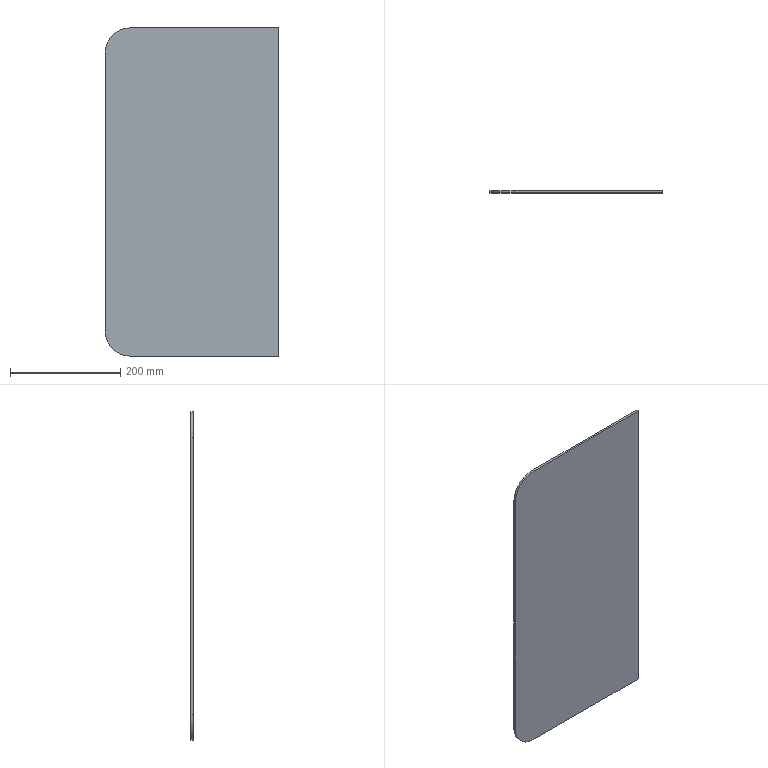Part | SolidWorks | features Extrusion 1 | 1 solid | 8 faces | box 315.5 x 4 x 596 mm | volume 748519 mm3 | plane 6 | cylinder 2 | commonest cylinder face diameters 92 x2
STEP:
#1=CARTESIAN_POINT('',(0.,0.,298.));
#2=VERTEX_POINT('',#1);
#3=CARTESIAN_POINT('',(0.,0.,-298.));
#4=VERTEX_POINT('',#3);
#5=CARTESIAN_POINT('',(0.,0.,-298.));
#6=DIRECTION('',(0.,0.,-1.));
#7=VECTOR('',#6,1000.);
#8=LINE('',#5,#7);
#9=EDGE_CURVE('',#2,#4,#8,.T.);
#10=ORIENTED_EDGE('',*,*,#9,.T.);
#11=CARTESIAN_POINT('',(0.,4.,-298.));
#12=VERTEX_POINT('',#11);
#13=CARTESIAN_POINT('',(0.,4.,-298.));
#14=DIRECTION('',(0.,-1.,0.));
#15=VECTOR('',#14,1000.);
#16=LINE('',#13,#15);
#17=EDGE_CURVE('',#12,#4,#16,.T.);
#18=ORIENTED_EDGE('',*,*,#17,.F.);
#19=CARTESIAN_POINT('',(0.,4.,298.));
#20=VERTEX_POINT('',#19);
#21=CARTESIAN_POINT('',(0.,4.,-298.));
#22=DIRECTION('',(0.,0.,-1.));
#23=VECTOR('',#22,1000.);
#24=LINE('',#21,#23);
#25=EDGE_CURVE('',#20,#12,#24,.T.);
#26=ORIENTED_EDGE('',*,*,#25,.F.);
#27=CARTESIAN_POINT('',(0.,4.,298.));
#28=DIRECTION('',(0.,-1.,0.));
#29=VECTOR('',#28,1000.);
#30=LINE('',#27,#29);
#31=EDGE_CURVE('',#20,#2,#30,.T.);
#32=ORIENTED_EDGE('',*,*,#31,.T.);
#33=EDGE_LOOP('',(#10,#18,#26,#32));
#34=FACE_OUTER_BOUND('',#33,.T.);
#35=CARTESIAN_POINT('',(0.,4.,-298.));
#36=DIRECTION('',(-1.,0.,0.));
#37=DIRECTION('',(0.,0.,1.));
#38=AXIS2_PLACEMENT_3D('',#35,#36,#37);
#39=PLANE('',#38);
#40=ADVANCED_FACE('',(#34),#39,.F.);
#41=CARTESIAN_POINT('',(-269.5,0.,-298.));
#42=VERTEX_POINT('',#41);
#43=CARTESIAN_POINT('',(0.,0.,-298.));
#44=DIRECTION('',(-1.,0.,0.));
#45=VECTOR('',#44,1000.);
#46=LINE('',#43,#45);
#47=EDGE_CURVE('',#4,#42,#46,.T.);
#48=ORIENTED_EDGE('',*,*,#47,.T.);
#49=CARTESIAN_POINT('',(-269.5,4.,-298.));
#50=VERTEX_POINT('',#49);
#51=CARTESIAN_POINT('',(-269.5,4.,-298.));
#52=DIRECTION('',(0.,-1.,0.));
#53=VECTOR('',#52,1000.);
#54=LINE('',#51,#53);
#55=EDGE_CURVE('',#50,#42,#54,.T.);
#56=ORIENTED_EDGE('',*,*,#55,.F.);
#57=CARTESIAN_POINT('',(0.,4.,-298.));
#58=DIRECTION('',(-1.,0.,0.));
#59=VECTOR('',#58,1000.);
#60=LINE('',#57,#59);
#61=EDGE_CURVE('',#12,#50,#60,.T.);
#62=ORIENTED_EDGE('',*,*,#61,.F.);
#63=ORIENTED_EDGE('',*,*,#17,.T.);
#64=EDGE_LOOP('',(#48,#56,#62,#63));
#65=FACE_OUTER_BOUND('',#64,.T.);
#66=CARTESIAN_POINT('',(0.,4.,-298.));
#67=DIRECTION('',(0.,0.,1.));
#68=DIRECTION('',(1.,0.,0.));
#69=AXIS2_PLACEMENT_3D('',#66,#67,#68);
#70=PLANE('',#69);
#71=ADVANCED_FACE('',(#65),#70,.F.);
#72=CARTESIAN_POINT('',(-315.5,0.,-252.));
#73=VERTEX_POINT('',#72);
#74=CARTESIAN_POINT('',(-269.5,0.,-252.));
#75=DIRECTION('',(0.,1.,0.));
#76=DIRECTION('',(0.,0.,1.));
#77=AXIS2_PLACEMENT_3D('',#74,#75,#76);
#78=CIRCLE('',#77,46.);
#79=EDGE_CURVE('',#42,#73,#78,.T.);
#80=ORIENTED_EDGE('',*,*,#79,.T.);
#81=CARTESIAN_POINT('',(-315.5,4.,-252.));
#82=VERTEX_POINT('',#81);
#83=CARTESIAN_POINT('',(-315.5,4.,-252.));
#84=DIRECTION('',(0.,-1.,0.));
#85=VECTOR('',#84,1000.);
#86=LINE('',#83,#85);
#87=EDGE_CURVE('',#82,#73,#86,.T.);
#88=ORIENTED_EDGE('',*,*,#87,.F.);
#89=CARTESIAN_POINT('',(-269.5,4.,-252.));
#90=DIRECTION('',(0.,1.,0.));
#91=DIRECTION('',(0.,0.,1.));
#92=AXIS2_PLACEMENT_3D('',#89,#90,#91);
#93=CIRCLE('',#92,46.);
#94=EDGE_CURVE('',#50,#82,#93,.T.);
#95=ORIENTED_EDGE('',*,*,#94,.F.);
#96=ORIENTED_EDGE('',*,*,#55,.T.);
#97=EDGE_LOOP('',(#80,#88,#95,#96));
#98=FACE_OUTER_BOUND('',#97,.T.);
#99=CARTESIAN_POINT('',(-269.5,4.,-252.));
#100=DIRECTION('',(0.,-1.,0.));
#101=DIRECTION('',(0.,0.,-1.));
#102=AXIS2_PLACEMENT_3D('',#99,#100,#101);
#103=CYLINDRICAL_SURFACE('',#102,46.);
#104=ADVANCED_FACE('',(#98),#103,.T.);
#105=CARTESIAN_POINT('',(-315.5,0.,252.));
#106=VERTEX_POINT('',#105);
#107=CARTESIAN_POINT('',(-315.5,0.,-252.));
#108=DIRECTION('',(0.,0.,1.));
#109=VECTOR('',#108,1000.);
#110=LINE('',#107,#109);
#111=EDGE_CURVE('',#73,#106,#110,.T.);
#112=ORIENTED_EDGE('',*,*,#111,.T.);
#113=CARTESIAN_POINT('',(-315.5,4.,252.));
#114=VERTEX_POINT('',#113);
#115=CARTESIAN_POINT('',(-315.5,4.,252.));
#116=DIRECTION('',(0.,-1.,0.));
#117=VECTOR('',#116,1000.);
#118=LINE('',#115,#117);
#119=EDGE_CURVE('',#114,#106,#118,.T.);
#120=ORIENTED_EDGE('',*,*,#119,.F.);
#121=CARTESIAN_POINT('',(-315.5,4.,-252.));
#122=DIRECTION('',(0.,0.,1.));
#123=VECTOR('',#122,1000.);
#124=LINE('',#121,#123);
#125=EDGE_CURVE('',#82,#114,#124,.T.);
#126=ORIENTED_EDGE('',*,*,#125,.F.);
#127=ORIENTED_EDGE('',*,*,#87,.T.);
#128=EDGE_LOOP('',(#112,#120,#126,#127));
#129=FACE_OUTER_BOUND('',#128,.T.);
#130=CARTESIAN_POINT('',(-315.5,4.,-252.));
#131=DIRECTION('',(1.,0.,0.));
#132=DIRECTION('',(0.,0.,-1.));
#133=AXIS2_PLACEMENT_3D('',#130,#131,#132);
#134=PLANE('',#133);
#135=ADVANCED_FACE('',(#129),#134,.F.);
#136=CARTESIAN_POINT('',(-269.5,0.,298.));
#137=VERTEX_POINT('',#136);
#138=CARTESIAN_POINT('',(-269.5,0.,252.));
#139=DIRECTION('',(0.,1.,0.));
#140=DIRECTION('',(0.,0.,1.));
#141=AXIS2_PLACEMENT_3D('',#138,#139,#140);
#142=CIRCLE('',#141,46.);
#143=EDGE_CURVE('',#106,#137,#142,.T.);
#144=ORIENTED_EDGE('',*,*,#143,.T.);
#145=CARTESIAN_POINT('',(-269.5,4.,298.));
#146=VERTEX_POINT('',#145);
#147=CARTESIAN_POINT('',(-269.5,4.,298.));
#148=DIRECTION('',(0.,-1.,0.));
#149=VECTOR('',#148,1000.);
#150=LINE('',#147,#149);
#151=EDGE_CURVE('',#146,#137,#150,.T.);
#152=ORIENTED_EDGE('',*,*,#151,.F.);
#153=CARTESIAN_POINT('',(-269.5,4.,252.));
#154=DIRECTION('',(0.,1.,0.));
#155=DIRECTION('',(0.,0.,1.));
#156=AXIS2_PLACEMENT_3D('',#153,#154,#155);
#157=CIRCLE('',#156,46.);
#158=EDGE_CURVE('',#114,#146,#157,.T.);
#159=ORIENTED_EDGE('',*,*,#158,.F.);
#160=ORIENTED_EDGE('',*,*,#119,.T.);
#161=EDGE_LOOP('',(#144,#152,#159,#160));
#162=FACE_OUTER_BOUND('',#161,.T.);
#163=CARTESIAN_POINT('',(-269.5,4.,252.));
#164=DIRECTION('',(0.,-1.,0.));
#165=DIRECTION('',(0.,0.,-1.));
#166=AXIS2_PLACEMENT_3D('',#163,#164,#165);
#167=CYLINDRICAL_SURFACE('',#166,46.);
#168=ADVANCED_FACE('',(#162),#167,.T.);
#169=CARTESIAN_POINT('',(-269.5,0.,298.));
#170=DIRECTION('',(1.,0.,0.));
#171=VECTOR('',#170,1000.);
#172=LINE('',#169,#171);
#173=EDGE_CURVE('',#137,#2,#172,.T.);
#174=ORIENTED_EDGE('',*,*,#173,.T.);
#175=ORIENTED_EDGE('',*,*,#31,.F.);
#176=CARTESIAN_POINT('',(-269.5,4.,298.));
#177=DIRECTION('',(1.,0.,0.));
#178=VECTOR('',#177,1000.);
#179=LINE('',#176,#178);
#180=EDGE_CURVE('',#146,#20,#179,.T.);
#181=ORIENTED_EDGE('',*,*,#180,.F.);
#182=ORIENTED_EDGE('',*,*,#151,.T.);
#183=EDGE_LOOP('',(#174,#175,#181,#182));
#184=FACE_OUTER_BOUND('',#183,.T.);
#185=CARTESIAN_POINT('',(-269.5,4.,298.));
#186=DIRECTION('',(0.,0.,-1.));
#187=DIRECTION('',(-1.,0.,0.));
#188=AXIS2_PLACEMENT_3D('',#185,#186,#187);
#189=PLANE('',#188);
#190=ADVANCED_FACE('',(#184),#189,.F.);
#191=ORIENTED_EDGE('',*,*,#25,.T.);
#192=ORIENTED_EDGE('',*,*,#61,.T.);
#193=ORIENTED_EDGE('',*,*,#94,.T.);
#194=ORIENTED_EDGE('',*,*,#125,.T.);
#195=ORIENTED_EDGE('',*,*,#158,.T.);
#196=ORIENTED_EDGE('',*,*,#180,.T.);
#197=EDGE_LOOP('',(#191,#192,#193,#194,#195,#196));
#198=FACE_OUTER_BOUND('',#197,.T.);
#199=CARTESIAN_POINT('',(-269.5,4.,252.));
#200=DIRECTION('',(0.,1.,0.));
#201=DIRECTION('',(0.,0.,1.));
#202=AXIS2_PLACEMENT_3D('',#199,#200,#201);
#203=PLANE('',#202);
#204=ADVANCED_FACE('',(#198),#203,.T.);
#205=ORIENTED_EDGE('',*,*,#9,.F.);
#206=ORIENTED_EDGE('',*,*,#173,.F.);
#207=ORIENTED_EDGE('',*,*,#143,.F.);
#208=ORIENTED_EDGE('',*,*,#111,.F.);
#209=ORIENTED_EDGE('',*,*,#79,.F.);
#210=ORIENTED_EDGE('',*,*,#47,.F.);
#211=EDGE_LOOP('',(#205,#206,#207,#208,#209,#210));
#212=FACE_OUTER_BOUND('',#211,.T.);
#213=CARTESIAN_POINT('',(-269.5,0.,252.));
#214=DIRECTION('',(0.,1.,0.));
#215=DIRECTION('',(0.,0.,1.));
#216=AXIS2_PLACEMENT_3D('',#213,#214,#215);
#217=PLANE('',#216);
#218=ADVANCED_FACE('',(#212),#217,.F.);
#219=CLOSED_SHELL('',(#40,#71,#104,#135,#168,#190,#204,#218));
#220=MANIFOLD_SOLID_BREP('',#219);
#221=CARTESIAN_POINT('',(0.,0.,0.));
#222=DIRECTION('',(0.,0.,1.));
#223=DIRECTION('',(1.,0.,0.));
#224=AXIS2_PLACEMENT_3D('',#221,#222,#223);
#225=(LENGTH_UNIT()NAMED_UNIT(*)SI_UNIT(.MILLI.,.METRE.));
#226=UNCERTAINTY_MEASURE_WITH_UNIT(LENGTH_MEASURE(0.00001),#225,'','');
#227=(NAMED_UNIT(*)PLANE_ANGLE_UNIT()SI_UNIT($,.RADIAN.));
#228=(NAMED_UNIT(*)SI_UNIT($,.STERADIAN.)SOLID_ANGLE_UNIT());
#229=(GEOMETRIC_REPRESENTATION_CONTEXT(3)GLOBAL_UNCERTAINTY_ASSIGNED_CONTEXT((#226))GLOBAL_UNIT_ASSIGNED_CONTEXT((#225,#227,#228))REPRESENTATION_CONTEXT('',''));
#230=ADVANCED_BREP_SHAPE_REPRESENTATION('',(#220,#224),#229);